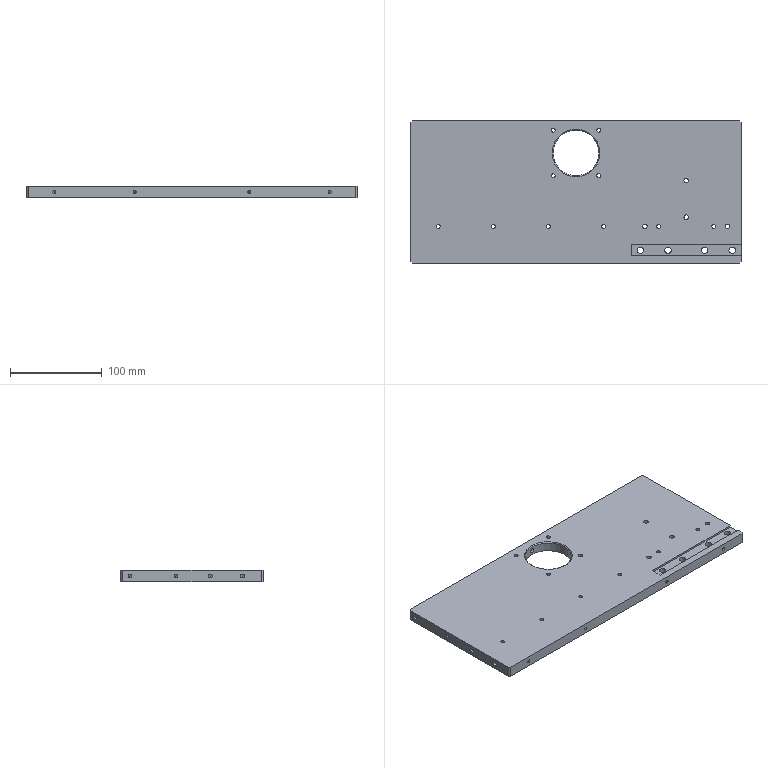CAM job | NX | 3-axis milling, drilling | part box 360 x 155 x 12 mm | stock box 364 x 155 x 12 mm
Tools:
number,name,description,diameter,corner_radius,flute_length,length,flutes
6,D8A45,Milling Tool-5 Parameters,8.0,0.0,50.0,75.0,2
13,4.2ZT,Drilling Tool,4.2,0.0,35.0,50.0,2
4,D10,Milling Tool-5 Parameters,10.0,0.0,50.0,75.0,2
22,7.0ZT,Drilling Tool,7.0,0.0,35.0,50.0,2
14,5.0ZT,Drilling Tool,5.0,0.0,35.0,50.0,2
Operations:
program,operation,operation_type,tool,method,geometry_group,spindle_rpm,surface_speed,feed_per_tooth,feed_cut,feed_plunge,cut_length_mm,path_length_mm,cut_time_min,machine_time_min
1压宽度,DRILLING,Operation,D8A45,METHOD,A,3500.0,65.0,0.0357,250.0,0.0,98.8,1094.19,0.3952,0.4947
1压宽度,DRILLING_1,Operation,4.2ZT,METHOD,A,2000.0,26.0,0.05,200.0,0.0,177.618,1022.463,0.8881,0.9726
1压宽度,DRILLING_1_COPY,Operation,7.0ZT,METHOD,A,2000.0,26.0,0.05,200.0,0.0,74.412,398.236,0.3721,0.4044
1压宽度,DRILLING_COPY,Operation,5.0ZT,METHOD,A,1500.0,15.0,0.05,150.0,0.0,72.009,446.66,0.4801,0.5175
1压宽度,HOLE_MILLING,CylinderMilling,D10,METHOD,A,7000.0,0.0,0.0,2000.0,100.0,3501.266,3677.766,1.751,1.768
1压宽度,HOLE_MILLING_COPY,CylinderMilling,D10,METHOD,A,7000.0,0.0,0.0857,1200.0,100.0,618.38,769.88,0.5153,0.5305
1压宽度,ZLEVEL_PROFILE_1,ZLevelMilling,D10,METHOD,A,7000.0,219.0,0.2143,3000.0,1000.0,4339.489,5063.825,1.487,1.56
1压宽度,ZLEVEL_PROFILE_1_COPY,ZLevelMilling,D10,METHOD,A,7000.0,219.0,0.2143,3000.0,1000.0,501.268,645.268,0.1725,0.1869
1压宽度,ZLEVEL_PROFILE_COPY_COPY,ZLevelMilling,D10,METHOD,A,7000.0,219.0,0.0714,1000.0,1000.0,470.685,1510.915,0.4707,0.5747
1压宽度,ZLEVEL_PROFILE_COPY_COPY_COPY,ZLevelMilling,D10,METHOD,A,7000.0,219.0,0.0714,1000.0,1000.0,239.664,383.664,0.2397,0.2541
1压宽度,PLANAR_MILL_COPY,PlanarMilling,D8A45,METHOD,A,7000.0,1495.0,0.0893,1250.0,100.0,338.966,3053.238,0.2712,0.5426
1压宽度,PLANAR_MILL_COPY_COPY,PlanarMilling,D8A45,METHOD,A,7000.0,1495.0,0.0893,1250.0,100.0,161.691,301.691,0.1294,0.1434